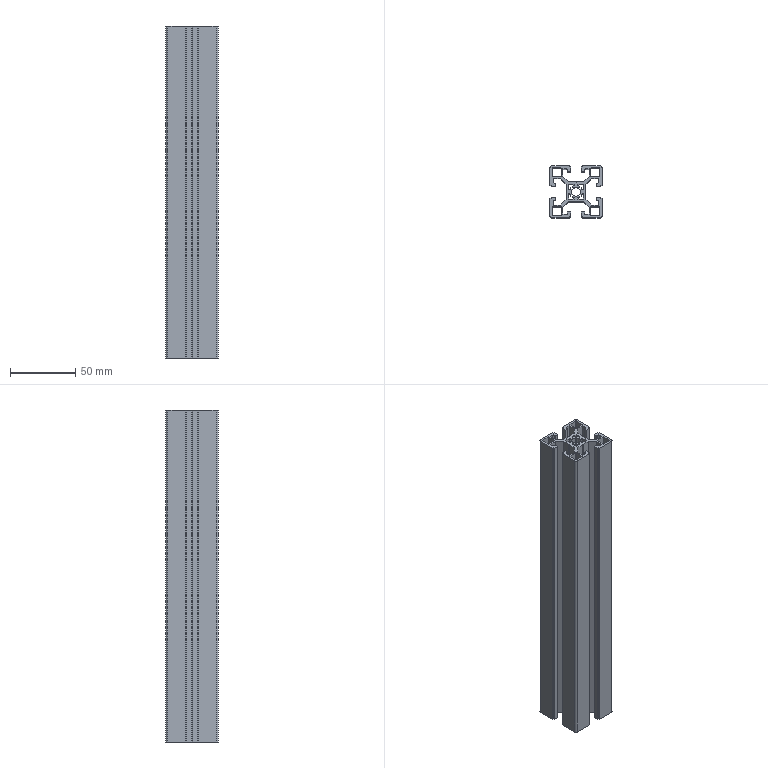Part | SolidWorks | features BaseBody 1, HoleWzd 1, MoveFace 1 | 1 solid | 179 faces | box 40 x 40 x 255 mm | volume 136655 mm3 | plane 130 | cylinder 49 | commonest cylinder face diameters 0.6 x24 2 x8 10 x8 6.8 x5 3 x4